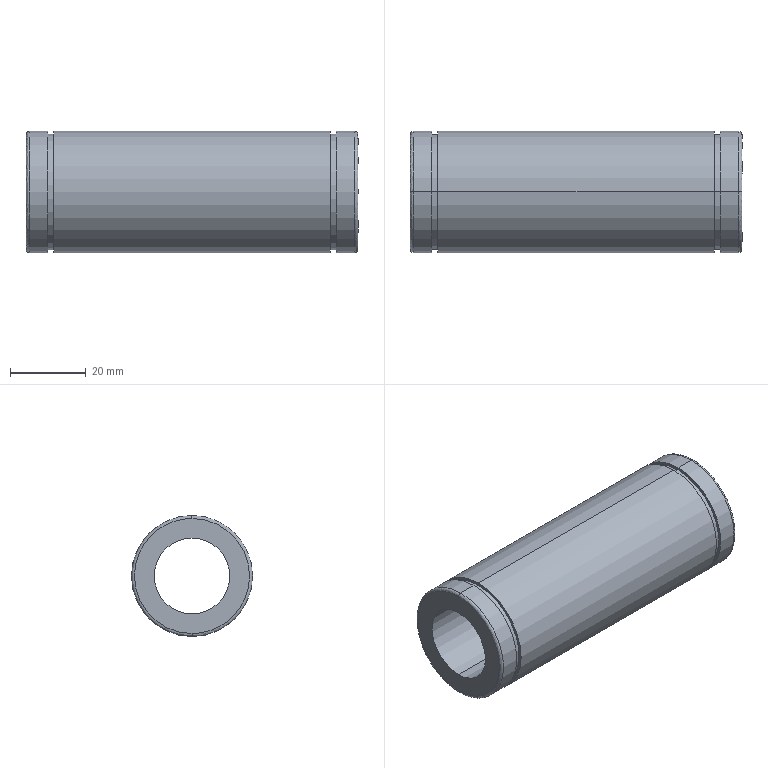Part | SolidWorks | features BaseBody 1 | 1 solid | 22 faces | box 87.7 x 32 x 32 mm | volume 42721 mm3 | cylinder 12 | plane 6 | spline 4 | commonest cylinder face diameters 32 x6 30.5 x4 20 x2
STEP:
#1=CARTESIAN_POINT('',(87.7,0.,-15.2));
#2=VERTEX_POINT('',#1);
#3=CARTESIAN_POINT('',(87.7,0.,15.2));
#4=VERTEX_POINT('',#3);
#5=CARTESIAN_POINT('',(87.7,0.,-15.2));
#6=CARTESIAN_POINT('',(87.7,-30.4,-15.2));
#7=CARTESIAN_POINT('',(87.7,-30.4,15.2));
#8=CARTESIAN_POINT('',(87.7,0.,15.2));
#9=(BOUNDED_CURVE()B_SPLINE_CURVE(3,(#5,#6,#7,#8),.UNSPECIFIED.,.F.,.F.)B_SPLINE_CURVE_WITH_KNOTS((4,4),(0.,0.5),.UNSPECIFIED.)CURVE()GEOMETRIC_REPRESENTATION_ITEM()RATIONAL_B_SPLINE_CURVE((1.,0.3333,0.3333,1.))REPRESENTATION_ITEM(''));
#10=EDGE_CURVE('',#2,#4,#9,.T.);
#11=ORIENTED_EDGE('',*,*,#10,.T.);
#12=CARTESIAN_POINT('',(86.9,0.,16.));
#13=VERTEX_POINT('',#12);
#14=CARTESIAN_POINT('',(86.9,0.,15.2));
#15=DIRECTION('',(0.,-1.,0.));
#16=DIRECTION('',(0.,0.,1.));
#17=AXIS2_PLACEMENT_3D('',#14,#15,#16);
#18=CIRCLE('',#17,0.8);
#19=EDGE_CURVE('',#4,#13,#18,.T.);
#20=ORIENTED_EDGE('',*,*,#19,.T.);
#21=CARTESIAN_POINT('',(86.9,0.,-16.));
#22=VERTEX_POINT('',#21);
#23=CARTESIAN_POINT('',(86.9,0.,0.));
#24=DIRECTION('',(-1.,0.,0.));
#25=DIRECTION('',(0.,0.,1.));
#26=AXIS2_PLACEMENT_3D('',#23,#24,#25);
#27=CIRCLE('',#26,16.);
#28=EDGE_CURVE('',#22,#13,#27,.T.);
#29=ORIENTED_EDGE('',*,*,#28,.F.);
#30=CARTESIAN_POINT('',(86.9,0.,-15.2));
#31=DIRECTION('',(0.,1.,0.));
#32=DIRECTION('',(0.,0.,-1.));
#33=AXIS2_PLACEMENT_3D('',#30,#31,#32);
#34=CIRCLE('',#33,0.8);
#35=EDGE_CURVE('',#2,#22,#34,.T.);
#36=ORIENTED_EDGE('',*,*,#35,.F.);
#37=EDGE_LOOP('',(#11,#20,#29,#36));
#38=FACE_OUTER_BOUND('',#37,.T.);
#39=CARTESIAN_POINT('',(87.7,0.,15.2));
#40=CARTESIAN_POINT('',(87.7,-30.4,15.2));
#41=CARTESIAN_POINT('',(87.7,-30.4,-15.2));
#42=CARTESIAN_POINT('',(87.7,0.,-15.2));
#43=CARTESIAN_POINT('',(87.7,0.,15.669));
#44=CARTESIAN_POINT('',(87.7,-31.337,15.669));
#45=CARTESIAN_POINT('',(87.7,-31.337,-15.669));
#46=CARTESIAN_POINT('',(87.7,0.,-15.669));
#47=CARTESIAN_POINT('',(87.369,0.,16.));
#48=CARTESIAN_POINT('',(87.369,-32.,16.));
#49=CARTESIAN_POINT('',(87.369,-32.,-16.));
#50=CARTESIAN_POINT('',(87.369,0.,-16.));
#51=CARTESIAN_POINT('',(86.9,0.,16.));
#52=CARTESIAN_POINT('',(86.9,-32.,16.));
#53=CARTESIAN_POINT('',(86.9,-32.,-16.));
#54=CARTESIAN_POINT('',(86.9,0.,-16.));
#55=(BOUNDED_SURFACE()B_SPLINE_SURFACE(3,3,((#39,#40,#41,#42),(#43,#44,#45,#46),(#47,#48,#49,#50),(#51,#52,#53,#54)),.UNSPECIFIED.,.F.,.F.,.F.)B_SPLINE_SURFACE_WITH_KNOTS((4,4),(4,4),(0.,1.),(0.,1.),.UNSPECIFIED.)GEOMETRIC_REPRESENTATION_ITEM()RATIONAL_B_SPLINE_SURFACE(((1.,0.3333,0.3333,1.),(0.8047,0.2682,0.2682,0.8047),(0.8047,0.2682,0.2682,0.8047),(1.,0.3333,0.3333,1.)))REPRESENTATION_ITEM('')SURFACE());
#56=ADVANCED_FACE('',(#38),#55,.T.);
#57=CARTESIAN_POINT('',(0.8,0.,16.));
#58=VERTEX_POINT('',#57);
#59=CARTESIAN_POINT('',(0.8,0.,-16.));
#60=VERTEX_POINT('',#59);
#61=CARTESIAN_POINT('',(0.8,0.,0.));
#62=DIRECTION('',(1.,0.,0.));
#63=DIRECTION('',(0.,0.,1.));
#64=AXIS2_PLACEMENT_3D('',#61,#62,#63);
#65=CIRCLE('',#64,16.);
#66=EDGE_CURVE('',#58,#60,#65,.T.);
#67=ORIENTED_EDGE('',*,*,#66,.F.);
#68=CARTESIAN_POINT('',(0.,0.,15.2));
#69=VERTEX_POINT('',#68);
#70=CARTESIAN_POINT('',(0.8,0.,15.2));
#71=DIRECTION('',(0.,-1.,0.));
#72=DIRECTION('',(0.,0.,1.));
#73=AXIS2_PLACEMENT_3D('',#70,#71,#72);
#74=CIRCLE('',#73,0.8);
#75=EDGE_CURVE('',#58,#69,#74,.T.);
#76=ORIENTED_EDGE('',*,*,#75,.T.);
#77=CARTESIAN_POINT('',(0.,0.,-15.2));
#78=VERTEX_POINT('',#77);
#79=CARTESIAN_POINT('',(0.,0.,15.2));
#80=CARTESIAN_POINT('',(0.,-30.4,15.2));
#81=CARTESIAN_POINT('',(0.,-30.4,-15.2));
#82=CARTESIAN_POINT('',(0.,0.,-15.2));
#83=(BOUNDED_CURVE()B_SPLINE_CURVE(3,(#79,#80,#81,#82),.UNSPECIFIED.,.F.,.F.)B_SPLINE_CURVE_WITH_KNOTS((4,4),(0.5,1.),.UNSPECIFIED.)CURVE()GEOMETRIC_REPRESENTATION_ITEM()RATIONAL_B_SPLINE_CURVE((1.,0.3333,0.3333,1.))REPRESENTATION_ITEM(''));
#84=EDGE_CURVE('',#69,#78,#83,.T.);
#85=ORIENTED_EDGE('',*,*,#84,.T.);
#86=CARTESIAN_POINT('',(0.8,0.,-15.2));
#87=DIRECTION('',(0.,1.,0.));
#88=DIRECTION('',(0.,0.,-1.));
#89=AXIS2_PLACEMENT_3D('',#86,#87,#88);
#90=CIRCLE('',#89,0.8);
#91=EDGE_CURVE('',#60,#78,#90,.T.);
#92=ORIENTED_EDGE('',*,*,#91,.F.);
#93=EDGE_LOOP('',(#67,#76,#85,#92));
#94=FACE_OUTER_BOUND('',#93,.T.);
#95=CARTESIAN_POINT('',(0.8,0.,16.));
#96=CARTESIAN_POINT('',(0.8,-32.,16.));
#97=CARTESIAN_POINT('',(0.8,-32.,-16.));
#98=CARTESIAN_POINT('',(0.8,0.,-16.));
#99=CARTESIAN_POINT('',(0.3314,0.,16.));
#100=CARTESIAN_POINT('',(0.3314,-32.,16.));
#101=CARTESIAN_POINT('',(0.3314,-32.,-16.));
#102=CARTESIAN_POINT('',(0.3314,0.,-16.));
#103=CARTESIAN_POINT('',(0.,0.,15.669));
#104=CARTESIAN_POINT('',(0.,-31.337,15.669));
#105=CARTESIAN_POINT('',(0.,-31.337,-15.669));
#106=CARTESIAN_POINT('',(0.,0.,-15.669));
#107=CARTESIAN_POINT('',(0.,0.,15.2));
#108=CARTESIAN_POINT('',(0.,-30.4,15.2));
#109=CARTESIAN_POINT('',(0.,-30.4,-15.2));
#110=CARTESIAN_POINT('',(0.,0.,-15.2));
#111=(BOUNDED_SURFACE()B_SPLINE_SURFACE(3,3,((#95,#96,#97,#98),(#99,#100,#101,#102),(#103,#104,#105,#106),(#107,#108,#109,#110)),.UNSPECIFIED.,.F.,.F.,.F.)B_SPLINE_SURFACE_WITH_KNOTS((4,4),(4,4),(0.,1.),(0.,1.),.UNSPECIFIED.)GEOMETRIC_REPRESENTATION_ITEM()RATIONAL_B_SPLINE_SURFACE(((1.,0.3333,0.3333,1.),(0.8047,0.2682,0.2682,0.8047),(0.8047,0.2682,0.2682,0.8047),(1.,0.3333,0.3333,1.)))REPRESENTATION_ITEM('')SURFACE());
#112=ADVANCED_FACE('',(#94),#111,.T.);
#113=CARTESIAN_POINT('',(80.35,0.,16.));
#114=VERTEX_POINT('',#113);
#115=CARTESIAN_POINT('',(80.35,0.,-16.));
#116=VERTEX_POINT('',#115);
#117=CARTESIAN_POINT('',(80.35,0.,0.));
#118=DIRECTION('',(-1.,0.,0.));
#119=DIRECTION('',(0.,0.,1.));
#120=AXIS2_PLACEMENT_3D('',#117,#118,#119);
#121=CIRCLE('',#120,16.);
#122=EDGE_CURVE('',#114,#116,#121,.T.);
#123=ORIENTED_EDGE('',*,*,#122,.T.);
#124=CARTESIAN_POINT('',(7.35,0.,-16.));
#125=VERTEX_POINT('',#124);
#126=CARTESIAN_POINT('',(87.7,0.,-16.));
#127=DIRECTION('',(-1.,0.,0.));
#128=VECTOR('',#127,1000.);
#129=LINE('',#126,#128);
#130=EDGE_CURVE('',#116,#125,#129,.T.);
#131=ORIENTED_EDGE('',*,*,#130,.T.);
#132=CARTESIAN_POINT('',(7.35,0.,16.));
#133=VERTEX_POINT('',#132);
#134=CARTESIAN_POINT('',(7.35,0.,0.));
#135=DIRECTION('',(1.,0.,0.));
#136=DIRECTION('',(0.,0.,1.));
#137=AXIS2_PLACEMENT_3D('',#134,#135,#136);
#138=CIRCLE('',#137,16.);
#139=EDGE_CURVE('',#125,#133,#138,.T.);
#140=ORIENTED_EDGE('',*,*,#139,.T.);
#141=CARTESIAN_POINT('',(87.7,0.,16.));
#142=DIRECTION('',(-1.,0.,0.));
#143=VECTOR('',#142,1000.);
#144=LINE('',#141,#143);
#145=EDGE_CURVE('',#114,#133,#144,.T.);
#146=ORIENTED_EDGE('',*,*,#145,.F.);
#147=EDGE_LOOP('',(#123,#131,#140,#146));
#148=FACE_OUTER_BOUND('',#147,.T.);
#149=CARTESIAN_POINT('',(87.7,0.,0.));
#150=DIRECTION('',(-1.,0.,0.));
#151=DIRECTION('',(0.,0.,1.));
#152=AXIS2_PLACEMENT_3D('',#149,#150,#151);
#153=CYLINDRICAL_SURFACE('',#152,16.);
#154=ADVANCED_FACE('',(#148),#153,.T.);
#155=CARTESIAN_POINT('',(81.95,0.,15.25));
#156=VERTEX_POINT('',#155);
#157=CARTESIAN_POINT('',(81.95,0.,-15.25));
#158=VERTEX_POINT('',#157);
#159=CARTESIAN_POINT('',(81.95,0.,0.));
#160=DIRECTION('',(-1.,0.,0.));
#161=DIRECTION('',(0.,0.,1.));
#162=AXIS2_PLACEMENT_3D('',#159,#160,#161);
#163=CIRCLE('',#162,15.25);
#164=EDGE_CURVE('',#156,#158,#163,.T.);
#165=ORIENTED_EDGE('',*,*,#164,.T.);
#166=CARTESIAN_POINT('',(80.35,0.,-15.25));
#167=VERTEX_POINT('',#166);
#168=CARTESIAN_POINT('',(87.7,0.,-15.25));
#169=DIRECTION('',(-1.,0.,0.));
#170=VECTOR('',#169,1000.);
#171=LINE('',#168,#170);
#172=EDGE_CURVE('',#158,#167,#171,.T.);
#173=ORIENTED_EDGE('',*,*,#172,.T.);
#174=CARTESIAN_POINT('',(80.35,0.,15.25));
#175=VERTEX_POINT('',#174);
#176=CARTESIAN_POINT('',(80.35,0.,0.));
#177=DIRECTION('',(-1.,0.,0.));
#178=DIRECTION('',(0.,0.,1.));
#179=AXIS2_PLACEMENT_3D('',#176,#177,#178);
#180=CIRCLE('',#179,15.25);
#181=EDGE_CURVE('',#175,#167,#180,.T.);
#182=ORIENTED_EDGE('',*,*,#181,.F.);
#183=CARTESIAN_POINT('',(87.7,0.,15.25));
#184=DIRECTION('',(-1.,0.,0.));
#185=VECTOR('',#184,1000.);
#186=LINE('',#183,#185);
#187=EDGE_CURVE('',#156,#175,#186,.T.);
#188=ORIENTED_EDGE('',*,*,#187,.F.);
#189=EDGE_LOOP('',(#165,#173,#182,#188));
#190=FACE_OUTER_BOUND('',#189,.T.);
#191=CARTESIAN_POINT('',(87.7,0.,0.));
#192=DIRECTION('',(-1.,0.,0.));
#193=DIRECTION('',(0.,0.,1.));
#194=AXIS2_PLACEMENT_3D('',#191,#192,#193);
#195=CYLINDRICAL_SURFACE('',#194,15.25);
#196=ADVANCED_FACE('',(#190),#195,.T.);
#197=CARTESIAN_POINT('',(7.35,0.,-15.25));
#198=VERTEX_POINT('',#197);
#199=CARTESIAN_POINT('',(7.35,0.,15.25));
#200=VERTEX_POINT('',#199);
#201=CARTESIAN_POINT('',(7.35,0.,0.));
#202=DIRECTION('',(1.,0.,0.));
#203=DIRECTION('',(0.,0.,1.));
#204=AXIS2_PLACEMENT_3D('',#201,#202,#203);
#205=CIRCLE('',#204,15.25);
#206=EDGE_CURVE('',#198,#200,#205,.T.);
#207=ORIENTED_EDGE('',*,*,#206,.F.);
#208=CARTESIAN_POINT('',(5.75,0.,-15.25));
#209=VERTEX_POINT('',#208);
#210=CARTESIAN_POINT('',(87.7,0.,-15.25));
#211=DIRECTION('',(-1.,0.,0.));
#212=VECTOR('',#211,1000.);
#213=LINE('',#210,#212);
#214=EDGE_CURVE('',#198,#209,#213,.T.);
#215=ORIENTED_EDGE('',*,*,#214,.T.);
#216=CARTESIAN_POINT('',(5.75,0.,15.25));
#217=VERTEX_POINT('',#216);
#218=CARTESIAN_POINT('',(5.75,0.,0.));
#219=DIRECTION('',(1.,0.,0.));
#220=DIRECTION('',(0.,0.,1.));
#221=AXIS2_PLACEMENT_3D('',#218,#219,#220);
#222=CIRCLE('',#221,15.25);
#223=EDGE_CURVE('',#209,#217,#222,.T.);
#224=ORIENTED_EDGE('',*,*,#223,.T.);
#225=CARTESIAN_POINT('',(87.7,0.,15.25));
#226=DIRECTION('',(-1.,0.,0.));
#227=VECTOR('',#226,1000.);
#228=LINE('',#225,#227);
#229=EDGE_CURVE('',#200,#217,#228,.T.);
#230=ORIENTED_EDGE('',*,*,#229,.F.);
#231=EDGE_LOOP('',(#207,#215,#224,#230));
#232=FACE_OUTER_BOUND('',#231,.T.);
#233=CARTESIAN_POINT('',(87.7,0.,0.));
#234=DIRECTION('',(-1.,0.,0.));
#235=DIRECTION('',(0.,0.,1.));
#236=AXIS2_PLACEMENT_3D('',#233,#234,#235);
#237=CYLINDRICAL_SURFACE('',#236,15.25);
#238=ADVANCED_FACE('',(#232),#237,.T.);
#239=CARTESIAN_POINT('',(86.9,0.,0.));
#240=DIRECTION('',(-1.,0.,0.));
#241=DIRECTION('',(0.,0.,1.));
#242=AXIS2_PLACEMENT_3D('',#239,#240,#241);
#243=CIRCLE('',#242,16.);
#244=EDGE_CURVE('',#13,#22,#243,.T.);
#245=ORIENTED_EDGE('',*,*,#244,.T.);
#246=CARTESIAN_POINT('',(81.95,0.,-16.));
#247=VERTEX_POINT('',#246);
#248=CARTESIAN_POINT('',(87.7,0.,-16.));
#249=DIRECTION('',(-1.,0.,0.));
#250=VECTOR('',#249,1000.);
#251=LINE('',#248,#250);
#252=EDGE_CURVE('',#22,#247,#251,.T.);
#253=ORIENTED_EDGE('',*,*,#252,.T.);
#254=CARTESIAN_POINT('',(81.95,0.,16.));
#255=VERTEX_POINT('',#254);
#256=CARTESIAN_POINT('',(81.95,0.,0.));
#257=DIRECTION('',(-1.,0.,0.));
#258=DIRECTION('',(0.,0.,1.));
#259=AXIS2_PLACEMENT_3D('',#256,#257,#258);
#260=CIRCLE('',#259,16.);
#261=EDGE_CURVE('',#255,#247,#260,.T.);
#262=ORIENTED_EDGE('',*,*,#261,.F.);
#263=CARTESIAN_POINT('',(87.7,0.,16.));
#264=DIRECTION('',(-1.,0.,0.));
#265=VECTOR('',#264,1000.);
#266=LINE('',#263,#265);
#267=EDGE_CURVE('',#13,#255,#266,.T.);
#268=ORIENTED_EDGE('',*,*,#267,.F.);
#269=EDGE_LOOP('',(#245,#253,#262,#268));
#270=FACE_OUTER_BOUND('',#269,.T.);
#271=CARTESIAN_POINT('',(87.7,0.,0.));
#272=DIRECTION('',(-1.,0.,0.));
#273=DIRECTION('',(0.,0.,1.));
#274=AXIS2_PLACEMENT_3D('',#271,#272,#273);
#275=CYLINDRICAL_SURFACE('',#274,16.);
#276=ADVANCED_FACE('',(#270),#275,.T.);
#277=CARTESIAN_POINT('',(5.75,0.,-16.));
#278=VERTEX_POINT('',#277);
#279=CARTESIAN_POINT('',(5.75,0.,16.));
#280=VERTEX_POINT('',#279);
#281=CARTESIAN_POINT('',(5.75,0.,0.));
#282=DIRECTION('',(1.,0.,0.));
#283=DIRECTION('',(0.,0.,1.));
#284=AXIS2_PLACEMENT_3D('',#281,#282,#283);
#285=CIRCLE('',#284,16.);
#286=EDGE_CURVE('',#278,#280,#285,.T.);
#287=ORIENTED_EDGE('',*,*,#286,.F.);
#288=CARTESIAN_POINT('',(87.7,0.,-16.));
#289=DIRECTION('',(-1.,0.,0.));
#290=VECTOR('',#289,1000.);
#291=LINE('',#288,#290);
#292=EDGE_CURVE('',#278,#60,#291,.T.);
#293=ORIENTED_EDGE('',*,*,#292,.T.);
#294=CARTESIAN_POINT('',(0.8,0.,0.));
#295=DIRECTION('',(1.,0.,0.));
#296=DIRECTION('',(0.,0.,1.));
#297=AXIS2_PLACEMENT_3D('',#294,#295,#296);
#298=CIRCLE('',#297,16.);
#299=EDGE_CURVE('',#60,#58,#298,.T.);
#300=ORIENTED_EDGE('',*,*,#299,.T.);
#301=CARTESIAN_POINT('',(87.7,0.,16.));
#302=DIRECTION('',(-1.,0.,0.));
#303=VECTOR('',#302,1000.);
#304=LINE('',#301,#303);
#305=EDGE_CURVE('',#280,#58,#304,.T.);
#306=ORIENTED_EDGE('',*,*,#305,.F.);
#307=EDGE_LOOP('',(#287,#293,#300,#306));
#308=FACE_OUTER_BOUND('',#307,.T.);
#309=CARTESIAN_POINT('',(87.7,0.,0.));
#310=DIRECTION('',(-1.,0.,0.));
#311=DIRECTION('',(0.,0.,1.));
#312=AXIS2_PLACEMENT_3D('',#309,#310,#311);
#313=CYLINDRICAL_SURFACE('',#312,16.);
#314=ADVANCED_FACE('',(#308),#313,.T.);
#315=CARTESIAN_POINT('',(87.7,0.,-10.));
#316=VERTEX_POINT('',#315);
#317=CARTESIAN_POINT('',(87.7,0.,10.));
#318=VERTEX_POINT('',#317);
#319=CARTESIAN_POINT('',(87.7,0.,0.));
#320=DIRECTION('',(-1.,0.,0.));
#321=DIRECTION('',(0.,0.,1.));
#322=AXIS2_PLACEMENT_3D('',#319,#320,#321);
#323=CIRCLE('',#322,10.);
#324=EDGE_CURVE('',#316,#318,#323,.T.);
#325=ORIENTED_EDGE('',*,*,#324,.F.);
#326=CARTESIAN_POINT('',(0.,0.,-10.));
#327=VERTEX_POINT('',#326);
#328=CARTESIAN_POINT('',(87.7,0.,-10.));
#329=DIRECTION('',(-1.,0.,0.));
#330=VECTOR('',#329,1000.);
#331=LINE('',#328,#330);
#332=EDGE_CURVE('',#316,#327,#331,.T.);
#333=ORIENTED_EDGE('',*,*,#332,.T.);
#334=CARTESIAN_POINT('',(0.,0.,10.));
#335=VERTEX_POINT('',#334);
#336=CARTESIAN_POINT('',(0.,0.,0.));
#337=DIRECTION('',(1.,0.,0.));
#338=DIRECTION('',(0.,0.,1.));
#339=AXIS2_PLACEMENT_3D('',#336,#337,#338);
#340=CIRCLE('',#339,10.);
#341=EDGE_CURVE('',#335,#327,#340,.T.);
#342=ORIENTED_EDGE('',*,*,#341,.F.);
#343=CARTESIAN_POINT('',(87.7,0.,10.));
#344=DIRECTION('',(-1.,0.,0.));
#345=VECTOR('',#344,1000.);
#346=LINE('',#343,#345);
#347=EDGE_CURVE('',#318,#335,#346,.T.);
#348=ORIENTED_EDGE('',*,*,#347,.F.);
#349=EDGE_LOOP('',(#325,#333,#342,#348));
#350=FACE_OUTER_BOUND('',#349,.T.);
#351=CARTESIAN_POINT('',(87.7,0.,0.));
#352=DIRECTION('',(-1.,0.,0.));
#353=DIRECTION('',(0.,0.,1.));
#354=AXIS2_PLACEMENT_3D('',#351,#352,#353);
#355=CYLINDRICAL_SURFACE('',#354,10.);
#356=ADVANCED_FACE('',(#350),#355,.F.);
#357=ORIENTED_EDGE('',*,*,#130,.F.);
#358=CARTESIAN_POINT('',(80.35,0.,0.));
#359=DIRECTION('',(-1.,0.,0.));
#360=DIRECTION('',(0.,0.,1.));
#361=AXIS2_PLACEMENT_3D('',#358,#359,#360);
#362=CIRCLE('',#361,16.);
#363=EDGE_CURVE('',#116,#114,#362,.T.);
#364=ORIENTED_EDGE('',*,*,#363,.T.);
#365=ORIENTED_EDGE('',*,*,#145,.T.);
#366=CARTESIAN_POINT('',(7.35,0.,0.));
#367=DIRECTION('',(1.,0.,0.));
#368=DIRECTION('',(0.,0.,1.));
#369=AXIS2_PLACEMENT_3D('',#366,#367,#368);
#370=CIRCLE('',#369,16.);
#371=EDGE_CURVE('',#133,#125,#370,.T.);
#372=ORIENTED_EDGE('',*,*,#371,.T.);
#373=EDGE_LOOP('',(#357,#364,#365,#372));
#374=FACE_OUTER_BOUND('',#373,.T.);
#375=CARTESIAN_POINT('',(87.7,0.,0.));
#376=DIRECTION('',(-1.,0.,0.));
#377=DIRECTION('',(0.,0.,1.));
#378=AXIS2_PLACEMENT_3D('',#375,#376,#377);
#379=CYLINDRICAL_SURFACE('',#378,16.);
#380=ADVANCED_FACE('',(#374),#379,.T.);
#381=ORIENTED_EDGE('',*,*,#181,.T.);
#382=CARTESIAN_POINT('',(80.35,0.,0.));
#383=DIRECTION('',(-1.,0.,0.));
#384=DIRECTION('',(0.,0.,1.));
#385=AXIS2_PLACEMENT_3D('',#382,#383,#384);
#386=CIRCLE('',#385,15.25);
#387=EDGE_CURVE('',#167,#175,#386,.T.);
#388=ORIENTED_EDGE('',*,*,#387,.T.);
#389=EDGE_LOOP('',(#381,#388));
#390=FACE_BOUND('',#389,.T.);
#391=ORIENTED_EDGE('',*,*,#122,.F.);
#392=ORIENTED_EDGE('',*,*,#363,.F.);
#393=EDGE_LOOP('',(#391,#392));
#394=FACE_OUTER_BOUND('',#393,.T.);
#395=CARTESIAN_POINT('',(80.35,15.25,0.));
#396=DIRECTION('',(1.,0.,0.));
#397=DIRECTION('',(0.,0.,-1.));
#398=AXIS2_PLACEMENT_3D('',#395,#396,#397);
#399=PLANE('',#398);
#400=ADVANCED_FACE('',(#390,#394),#399,.T.);
#401=ORIENTED_EDGE('',*,*,#371,.F.);
#402=ORIENTED_EDGE('',*,*,#139,.F.);
#403=EDGE_LOOP('',(#401,#402));
#404=FACE_OUTER_BOUND('',#403,.T.);
#405=CARTESIAN_POINT('',(7.35,0.,0.));
#406=DIRECTION('',(1.,0.,0.));
#407=DIRECTION('',(0.,0.,1.));
#408=AXIS2_PLACEMENT_3D('',#405,#406,#407);
#409=CIRCLE('',#408,15.25);
#410=EDGE_CURVE('',#200,#198,#409,.T.);
#411=ORIENTED_EDGE('',*,*,#410,.T.);
#412=ORIENTED_EDGE('',*,*,#206,.T.);
#413=EDGE_LOOP('',(#411,#412));
#414=FACE_BOUND('',#413,.T.);
#415=CARTESIAN_POINT('',(7.35,16.,0.));
#416=DIRECTION('',(-1.,0.,0.));
#417=DIRECTION('',(0.,0.,1.));
#418=AXIS2_PLACEMENT_3D('',#415,#416,#417);
#419=PLANE('',#418);
#420=ADVANCED_FACE('',(#404,#414),#419,.T.);
#421=ORIENTED_EDGE('',*,*,#172,.F.);
#422=CARTESIAN_POINT('',(81.95,0.,0.));
#423=DIRECTION('',(-1.,0.,0.));
#424=DIRECTION('',(0.,0.,1.));
#425=AXIS2_PLACEMENT_3D('',#422,#423,#424);
#426=CIRCLE('',#425,15.25);
#427=EDGE_CURVE('',#158,#156,#426,.T.);
#428=ORIENTED_EDGE('',*,*,#427,.T.);
#429=ORIENTED_EDGE('',*,*,#187,.T.);
#430=ORIENTED_EDGE('',*,*,#387,.F.);
#431=EDGE_LOOP('',(#421,#428,#429,#430));
#432=FACE_OUTER_BOUND('',#431,.T.);
#433=CARTESIAN_POINT('',(87.7,0.,0.));
#434=DIRECTION('',(-1.,0.,0.));
#435=DIRECTION('',(0.,0.,1.));
#436=AXIS2_PLACEMENT_3D('',#433,#434,#435);
#437=CYLINDRICAL_SURFACE('',#436,15.25);
#438=ADVANCED_FACE('',(#432),#437,.T.);
#439=ORIENTED_EDGE('',*,*,#214,.F.);
#440=ORIENTED_EDGE('',*,*,#410,.F.);
#441=ORIENTED_EDGE('',*,*,#229,.T.);
#442=CARTESIAN_POINT('',(5.75,0.,0.));
#443=DIRECTION('',(1.,0.,0.));
#444=DIRECTION('',(0.,0.,1.));
#445=AXIS2_PLACEMENT_3D('',#442,#443,#444);
#446=CIRCLE('',#445,15.25);
#447=EDGE_CURVE('',#217,#209,#446,.T.);
#448=ORIENTED_EDGE('',*,*,#447,.T.);
#449=EDGE_LOOP('',(#439,#440,#441,#448));
#450=FACE_OUTER_BOUND('',#449,.T.);
#451=CARTESIAN_POINT('',(87.7,0.,0.));
#452=DIRECTION('',(-1.,0.,0.));
#453=DIRECTION('',(0.,0.,1.));
#454=AXIS2_PLACEMENT_3D('',#451,#452,#453);
#455=CYLINDRICAL_SURFACE('',#454,15.25);
#456=ADVANCED_FACE('',(#450),#455,.T.);
#457=ORIENTED_EDGE('',*,*,#261,.T.);
#458=CARTESIAN_POINT('',(81.95,0.,0.));
#459=DIRECTION('',(-1.,0.,0.));
#460=DIRECTION('',(0.,0.,1.));
#461=AXIS2_PLACEMENT_3D('',#458,#459,#460);
#462=CIRCLE('',#461,16.);
#463=EDGE_CURVE('',#247,#255,#462,.T.);
#464=ORIENTED_EDGE('',*,*,#463,.T.);
#465=EDGE_LOOP('',(#457,#464));
#466=FACE_OUTER_BOUND('',#465,.T.);
#467=ORIENTED_EDGE('',*,*,#164,.F.);
#468=ORIENTED_EDGE('',*,*,#427,.F.);
#469=EDGE_LOOP('',(#467,#468));
#470=FACE_BOUND('',#469,.T.);
#471=CARTESIAN_POINT('',(81.95,16.,0.));
#472=DIRECTION('',(-1.,0.,0.));
#473=DIRECTION('',(0.,0.,1.));
#474=AXIS2_PLACEMENT_3D('',#471,#472,#473);
#475=PLANE('',#474);
#476=ADVANCED_FACE('',(#466,#470),#475,.T.);
#477=ORIENTED_EDGE('',*,*,#447,.F.);
#478=ORIENTED_EDGE('',*,*,#223,.F.);
#479=EDGE_LOOP('',(#477,#478));
#480=FACE_BOUND('',#479,.T.);
#481=CARTESIAN_POINT('',(5.75,0.,0.));
#482=DIRECTION('',(1.,0.,0.));
#483=DIRECTION('',(0.,0.,1.));
#484=AXIS2_PLACEMENT_3D('',#481,#482,#483);
#485=CIRCLE('',#484,16.);
#486=EDGE_CURVE('',#280,#278,#485,.T.);
#487=ORIENTED_EDGE('',*,*,#486,.T.);
#488=ORIENTED_EDGE('',*,*,#286,.T.);
#489=EDGE_LOOP('',(#487,#488));
#490=FACE_OUTER_BOUND('',#489,.T.);
#491=CARTESIAN_POINT('',(5.75,15.25,0.));
#492=DIRECTION('',(1.,0.,0.));
#493=DIRECTION('',(0.,0.,-1.));
#494=AXIS2_PLACEMENT_3D('',#491,#492,#493);
#495=PLANE('',#494);
#496=ADVANCED_FACE('',(#480,#490),#495,.T.);
#497=ORIENTED_EDGE('',*,*,#252,.F.);
#498=ORIENTED_EDGE('',*,*,#28,.T.);
#499=ORIENTED_EDGE('',*,*,#267,.T.);
#500=ORIENTED_EDGE('',*,*,#463,.F.);
#501=EDGE_LOOP('',(#497,#498,#499,#500));
#502=FACE_OUTER_BOUND('',#501,.T.);
#503=CARTESIAN_POINT('',(87.7,0.,0.));
#504=DIRECTION('',(-1.,0.,0.));
#505=DIRECTION('',(0.,0.,1.));
#506=AXIS2_PLACEMENT_3D('',#503,#504,#505);
#507=CYLINDRICAL_SURFACE('',#506,16.);
#508=ADVANCED_FACE('',(#502),#507,.T.);
#509=ORIENTED_EDGE('',*,*,#292,.F.);
#510=ORIENTED_EDGE('',*,*,#486,.F.);
#511=ORIENTED_EDGE('',*,*,#305,.T.);
#512=ORIENTED_EDGE('',*,*,#66,.T.);
#513=EDGE_LOOP('',(#509,#510,#511,#512));
#514=FACE_OUTER_BOUND('',#513,.T.);
#515=CARTESIAN_POINT('',(87.7,0.,0.));
#516=DIRECTION('',(-1.,0.,0.));
#517=DIRECTION('',(0.,0.,1.));
#518=AXIS2_PLACEMENT_3D('',#515,#516,#517);
#519=CYLINDRICAL_SURFACE('',#518,16.);
#520=ADVANCED_FACE('',(#514),#519,.T.);
#521=ORIENTED_EDGE('',*,*,#19,.F.);
#522=CARTESIAN_POINT('',(87.7,0.,15.2));
#523=CARTESIAN_POINT('',(87.7,30.4,15.2));
#524=CARTESIAN_POINT('',(87.7,30.4,-15.2));
#525=CARTESIAN_POINT('',(87.7,0.,-15.2));
#526=(BOUNDED_CURVE()B_SPLINE_CURVE(3,(#522,#523,#524,#525),.UNSPECIFIED.,.F.,.F.)B_SPLINE_CURVE_WITH_KNOTS((4,4),(0.5,1.),.UNSPECIFIED.)CURVE()GEOMETRIC_REPRESENTATION_ITEM()RATIONAL_B_SPLINE_CURVE((1.,0.3333,0.3333,1.))REPRESENTATION_ITEM(''));
#527=EDGE_CURVE('',#4,#2,#526,.T.);
#528=ORIENTED_EDGE('',*,*,#527,.T.);
#529=ORIENTED_EDGE('',*,*,#35,.T.);
#530=ORIENTED_EDGE('',*,*,#244,.F.);
#531=EDGE_LOOP('',(#521,#528,#529,#530));
#532=FACE_OUTER_BOUND('',#531,.T.);
#533=CARTESIAN_POINT('',(87.7,0.,-15.2));
#534=CARTESIAN_POINT('',(87.7,30.4,-15.2));
#535=CARTESIAN_POINT('',(87.7,30.4,15.2));
#536=CARTESIAN_POINT('',(87.7,0.,15.2));
#537=CARTESIAN_POINT('',(87.7,0.,-15.669));
#538=CARTESIAN_POINT('',(87.7,31.337,-15.669));
#539=CARTESIAN_POINT('',(87.7,31.337,15.669));
#540=CARTESIAN_POINT('',(87.7,0.,15.669));
#541=CARTESIAN_POINT('',(87.369,0.,-16.));
#542=CARTESIAN_POINT('',(87.369,32.,-16.));
#543=CARTESIAN_POINT('',(87.369,32.,16.));
#544=CARTESIAN_POINT('',(87.369,0.,16.));
#545=CARTESIAN_POINT('',(86.9,0.,-16.));
#546=CARTESIAN_POINT('',(86.9,32.,-16.));
#547=CARTESIAN_POINT('',(86.9,32.,16.));
#548=CARTESIAN_POINT('',(86.9,0.,16.));
#549=(BOUNDED_SURFACE()B_SPLINE_SURFACE(3,3,((#533,#534,#535,#536),(#537,#538,#539,#540),(#541,#542,#543,#544),(#545,#546,#547,#548)),.UNSPECIFIED.,.F.,.F.,.T.)B_SPLINE_SURFACE_WITH_KNOTS((4,4),(4,4),(0.,1.),(0.,1.),.UNSPECIFIED.)GEOMETRIC_REPRESENTATION_ITEM()RATIONAL_B_SPLINE_SURFACE(((1.,0.3333,0.3333,1.),(0.8047,0.2682,0.2682,0.8047),(0.8047,0.2682,0.2682,0.8047),(1.,0.3333,0.3333,1.)))REPRESENTATION_ITEM('')SURFACE());
#550=ADVANCED_FACE('',(#532),#549,.T.);
#551=ORIENTED_EDGE('',*,*,#75,.F.);
#552=ORIENTED_EDGE('',*,*,#299,.F.);
#553=ORIENTED_EDGE('',*,*,#91,.T.);
#554=CARTESIAN_POINT('',(0.,0.,-15.2));
#555=CARTESIAN_POINT('',(0.,30.4,-15.2));
#556=CARTESIAN_POINT('',(0.,30.4,15.2));
#557=CARTESIAN_POINT('',(0.,0.,15.2));
#558=(BOUNDED_CURVE()B_SPLINE_CURVE(3,(#554,#555,#556,#557),.UNSPECIFIED.,.F.,.F.)B_SPLINE_CURVE_WITH_KNOTS((4,4),(0.,0.5),.UNSPECIFIED.)CURVE()GEOMETRIC_REPRESENTATION_ITEM()RATIONAL_B_SPLINE_CURVE((1.,0.3333,0.3333,1.))REPRESENTATION_ITEM(''));
#559=EDGE_CURVE('',#78,#69,#558,.T.);
#560=ORIENTED_EDGE('',*,*,#559,.T.);
#561=EDGE_LOOP('',(#551,#552,#553,#560));
#562=FACE_OUTER_BOUND('',#561,.T.);
#563=CARTESIAN_POINT('',(0.8,0.,-16.));
#564=CARTESIAN_POINT('',(0.8,32.,-16.));
#565=CARTESIAN_POINT('',(0.8,32.,16.));
#566=CARTESIAN_POINT('',(0.8,0.,16.));
#567=CARTESIAN_POINT('',(0.3314,0.,-16.));
#568=CARTESIAN_POINT('',(0.3314,32.,-16.));
#569=CARTESIAN_POINT('',(0.3314,32.,16.));
#570=CARTESIAN_POINT('',(0.3314,0.,16.));
#571=CARTESIAN_POINT('',(0.,0.,-15.669));
#572=CARTESIAN_POINT('',(0.,31.337,-15.669));
#573=CARTESIAN_POINT('',(0.,31.337,15.669));
#574=CARTESIAN_POINT('',(0.,0.,15.669));
#575=CARTESIAN_POINT('',(0.,0.,-15.2));
#576=CARTESIAN_POINT('',(0.,30.4,-15.2));
#577=CARTESIAN_POINT('',(0.,30.4,15.2));
#578=CARTESIAN_POINT('',(0.,0.,15.2));
#579=(BOUNDED_SURFACE()B_SPLINE_SURFACE(3,3,((#563,#564,#565,#566),(#567,#568,#569,#570),(#571,#572,#573,#574),(#575,#576,#577,#578)),.UNSPECIFIED.,.F.,.F.,.F.)B_SPLINE_SURFACE_WITH_KNOTS((4,4),(4,4),(0.,1.),(0.,1.),.UNSPECIFIED.)GEOMETRIC_REPRESENTATION_ITEM()RATIONAL_B_SPLINE_SURFACE(((1.,0.3333,0.3333,1.),(0.8047,0.2682,0.2682,0.8047),(0.8047,0.2682,0.2682,0.8047),(1.,0.3333,0.3333,1.)))REPRESENTATION_ITEM('')SURFACE());
#580=ADVANCED_FACE('',(#562),#579,.T.);
#581=CARTESIAN_POINT('',(87.7,0.,0.));
#582=DIRECTION('',(-1.,0.,0.));
#583=DIRECTION('',(0.,0.,1.));
#584=AXIS2_PLACEMENT_3D('',#581,#582,#583);
#585=CIRCLE('',#584,10.);
#586=EDGE_CURVE('',#318,#316,#585,.T.);
#587=ORIENTED_EDGE('',*,*,#586,.T.);
#588=ORIENTED_EDGE('',*,*,#324,.T.);
#589=EDGE_LOOP('',(#587,#588));
#590=FACE_BOUND('',#589,.T.);
#591=ORIENTED_EDGE('',*,*,#10,.F.);
#592=ORIENTED_EDGE('',*,*,#527,.F.);
#593=EDGE_LOOP('',(#591,#592));
#594=FACE_OUTER_BOUND('',#593,.T.);
#595=CARTESIAN_POINT('',(87.7,10.,0.));
#596=DIRECTION('',(1.,0.,0.));
#597=DIRECTION('',(0.,0.,-1.));
#598=AXIS2_PLACEMENT_3D('',#595,#596,#597);
#599=PLANE('',#598);
#600=ADVANCED_FACE('',(#590,#594),#599,.T.);
#601=ORIENTED_EDGE('',*,*,#559,.F.);
#602=ORIENTED_EDGE('',*,*,#84,.F.);
#603=EDGE_LOOP('',(#601,#602));
#604=FACE_OUTER_BOUND('',#603,.T.);
#605=ORIENTED_EDGE('',*,*,#341,.T.);
#606=CARTESIAN_POINT('',(0.,0.,0.));
#607=DIRECTION('',(1.,0.,0.));
#608=DIRECTION('',(0.,0.,1.));
#609=AXIS2_PLACEMENT_3D('',#606,#607,#608);
#610=CIRCLE('',#609,10.);
#611=EDGE_CURVE('',#327,#335,#610,.T.);
#612=ORIENTED_EDGE('',*,*,#611,.T.);
#613=EDGE_LOOP('',(#605,#612));
#614=FACE_BOUND('',#613,.T.);
#615=CARTESIAN_POINT('',(0.,15.2,0.));
#616=DIRECTION('',(-1.,0.,0.));
#617=DIRECTION('',(0.,0.,1.));
#618=AXIS2_PLACEMENT_3D('',#615,#616,#617);
#619=PLANE('',#618);
#620=ADVANCED_FACE('',(#604,#614),#619,.T.);
#621=ORIENTED_EDGE('',*,*,#332,.F.);
#622=ORIENTED_EDGE('',*,*,#586,.F.);
#623=ORIENTED_EDGE('',*,*,#347,.T.);
#624=ORIENTED_EDGE('',*,*,#611,.F.);
#625=EDGE_LOOP('',(#621,#622,#623,#624));
#626=FACE_OUTER_BOUND('',#625,.T.);
#627=CARTESIAN_POINT('',(87.7,0.,0.));
#628=DIRECTION('',(-1.,0.,0.));
#629=DIRECTION('',(0.,0.,1.));
#630=AXIS2_PLACEMENT_3D('',#627,#628,#629);
#631=CYLINDRICAL_SURFACE('',#630,10.);
#632=ADVANCED_FACE('',(#626),#631,.F.);
#633=CLOSED_SHELL('',(#56,#112,#154,#196,#238,#276,#314,#356,#380,#400,#420,#438,#456,#476,#496,#508,#520,#550,#580,#600,#620,#632));
#634=MANIFOLD_SOLID_BREP('',#633);
#635=CARTESIAN_POINT('',(0.,0.,0.));
#636=DIRECTION('',(0.,0.,1.));
#637=DIRECTION('',(1.,0.,0.));
#638=AXIS2_PLACEMENT_3D('',#635,#636,#637);
#639=(LENGTH_UNIT()NAMED_UNIT(*)SI_UNIT(.MILLI.,.METRE.));
#640=UNCERTAINTY_MEASURE_WITH_UNIT(LENGTH_MEASURE(0.00001),#639,'','');
#641=(NAMED_UNIT(*)PLANE_ANGLE_UNIT()SI_UNIT($,.RADIAN.));
#642=(NAMED_UNIT(*)SI_UNIT($,.STERADIAN.)SOLID_ANGLE_UNIT());
#643=(GEOMETRIC_REPRESENTATION_CONTEXT(3)GLOBAL_UNCERTAINTY_ASSIGNED_CONTEXT((#640))GLOBAL_UNIT_ASSIGNED_CONTEXT((#639,#641,#642))REPRESENTATION_CONTEXT('',''));
#644=ADVANCED_BREP_SHAPE_REPRESENTATION('',(#634,#638),#643);